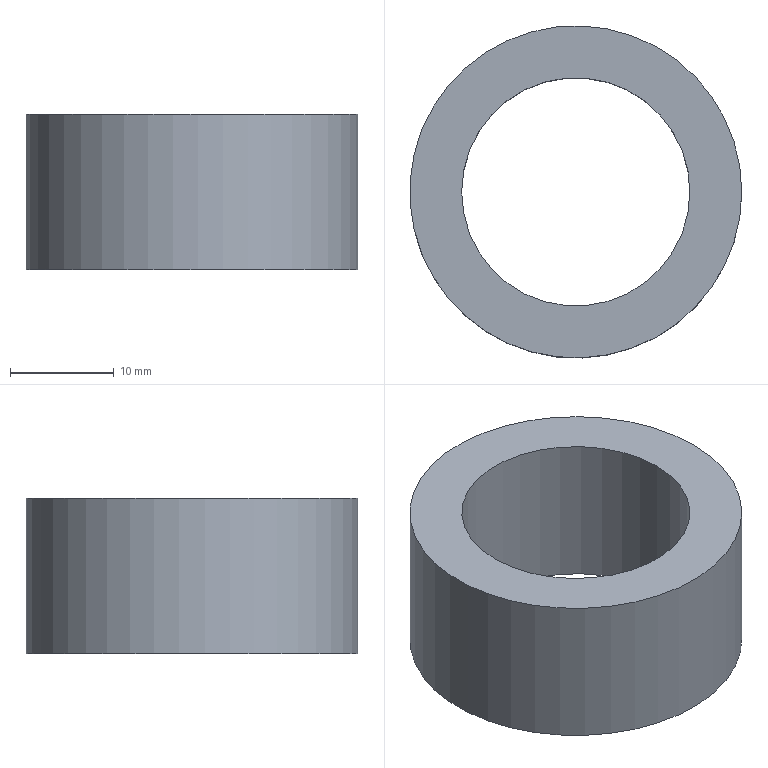Part | NX | features solid 2 | 1 solid | 4 faces | box 32 x 32 x 15 mm | volume 6362 mm3 | cylinder 2 | plane 2 | commonest cylinder face diameters 22 x1 32 x1
STEP:
#1=CARTESIAN_POINT('',(2071.861,45.692,86.));
#2=VERTEX_POINT('',#1);
#3=CARTESIAN_POINT('',(2055.861,45.692,86.));
#4=DIRECTION('',(0.,0.,-1.));
#5=DIRECTION('',(1.,0.,0.));
#6=AXIS2_PLACEMENT_3D('',#3,#4,#5);
#7=CIRCLE('',#6,16.);
#8=EDGE_CURVE('',#2,#2,#7,.T.);
#9=ORIENTED_EDGE('',*,*,#8,.F.);
#10=EDGE_LOOP('',(#9));
#11=FACE_BOUND('',#10,.T.);
#12=CARTESIAN_POINT('',(2071.861,45.692,101.));
#13=VERTEX_POINT('',#12);
#14=CARTESIAN_POINT('',(2055.861,45.692,101.));
#15=DIRECTION('',(0.,0.,-1.));
#16=DIRECTION('',(1.,0.,0.));
#17=AXIS2_PLACEMENT_3D('',#14,#15,#16);
#18=CIRCLE('',#17,16.);
#19=EDGE_CURVE('',#13,#13,#18,.T.);
#20=ORIENTED_EDGE('',*,*,#19,.T.);
#21=EDGE_LOOP('',(#20));
#22=FACE_BOUND('',#21,.T.);
#23=CARTESIAN_POINT('',(2055.861,45.692,84.5));
#24=DIRECTION('',(0.,0.,-1.));
#25=DIRECTION('',(-1.,0.,0.));
#26=AXIS2_PLACEMENT_3D('',#23,#24,#25);
#27=CYLINDRICAL_SURFACE('',#26,16.);
#28=ADVANCED_FACE('',(#11,#22),#27,.T.);
#29=CARTESIAN_POINT('',(2066.861,45.692,86.));
#30=VERTEX_POINT('',#29);
#31=CARTESIAN_POINT('',(2055.861,45.692,86.));
#32=DIRECTION('',(0.,0.,1.));
#33=DIRECTION('',(1.,0.,0.));
#34=AXIS2_PLACEMENT_3D('',#31,#32,#33);
#35=CIRCLE('',#34,11.);
#36=EDGE_CURVE('',#30,#30,#35,.T.);
#37=ORIENTED_EDGE('',*,*,#36,.F.);
#38=EDGE_LOOP('',(#37));
#39=FACE_BOUND('',#38,.T.);
#40=CARTESIAN_POINT('',(2066.861,45.692,101.));
#41=VERTEX_POINT('',#40);
#42=CARTESIAN_POINT('',(2055.861,45.692,101.));
#43=DIRECTION('',(0.,0.,1.));
#44=DIRECTION('',(1.,0.,0.));
#45=AXIS2_PLACEMENT_3D('',#42,#43,#44);
#46=CIRCLE('',#45,11.);
#47=EDGE_CURVE('',#41,#41,#46,.T.);
#48=ORIENTED_EDGE('',*,*,#47,.T.);
#49=EDGE_LOOP('',(#48));
#50=FACE_BOUND('',#49,.T.);
#51=CARTESIAN_POINT('',(2055.861,45.692,101.));
#52=DIRECTION('',(0.,0.,-1.));
#53=DIRECTION('',(1.,0.,0.));
#54=AXIS2_PLACEMENT_3D('',#51,#52,#53);
#55=CYLINDRICAL_SURFACE('',#54,11.);
#56=ADVANCED_FACE('',(#39,#50),#55,.F.);
#57=ORIENTED_EDGE('',*,*,#19,.F.);
#58=EDGE_LOOP('',(#57));
#59=FACE_BOUND('',#58,.T.);
#60=ORIENTED_EDGE('',*,*,#47,.F.);
#61=EDGE_LOOP('',(#60));
#62=FACE_BOUND('',#61,.T.);
#63=CARTESIAN_POINT('',(2055.861,45.692,101.));
#64=DIRECTION('',(0.,0.,1.));
#65=DIRECTION('',(1.,0.,0.));
#66=AXIS2_PLACEMENT_3D('',#63,#64,#65);
#67=PLANE('',#66);
#68=ADVANCED_FACE('',(#59,#62),#67,.T.);
#69=ORIENTED_EDGE('',*,*,#8,.T.);
#70=EDGE_LOOP('',(#69));
#71=FACE_BOUND('',#70,.T.);
#72=ORIENTED_EDGE('',*,*,#36,.T.);
#73=EDGE_LOOP('',(#72));
#74=FACE_BOUND('',#73,.T.);
#75=CARTESIAN_POINT('',(2055.861,45.692,86.));
#76=DIRECTION('',(0.,0.,1.));
#77=DIRECTION('',(1.,0.,0.));
#78=AXIS2_PLACEMENT_3D('',#75,#76,#77);
#79=PLANE('',#78);
#80=ADVANCED_FACE('',(#71,#74),#79,.F.);
#81=CLOSED_SHELL('',(#28,#56,#68,#80));
#82=MANIFOLD_SOLID_BREP('',#81);
#83=(LENGTH_UNIT()NAMED_UNIT(*)SI_UNIT(.MILLI.,.METRE.));
#84=UNCERTAINTY_MEASURE_WITH_UNIT(LENGTH_MEASURE(0.00001),#83,'','');
#85=(NAMED_UNIT(*)PLANE_ANGLE_UNIT()SI_UNIT($,.RADIAN.));
#86=(NAMED_UNIT(*)SI_UNIT($,.STERADIAN.)SOLID_ANGLE_UNIT());
#87=(GEOMETRIC_REPRESENTATION_CONTEXT(3)GLOBAL_UNCERTAINTY_ASSIGNED_CONTEXT((#84))GLOBAL_UNIT_ASSIGNED_CONTEXT((#83,#85,#86))REPRESENTATION_CONTEXT('',''));
#88=ADVANCED_BREP_SHAPE_REPRESENTATION('',(#82),#87);